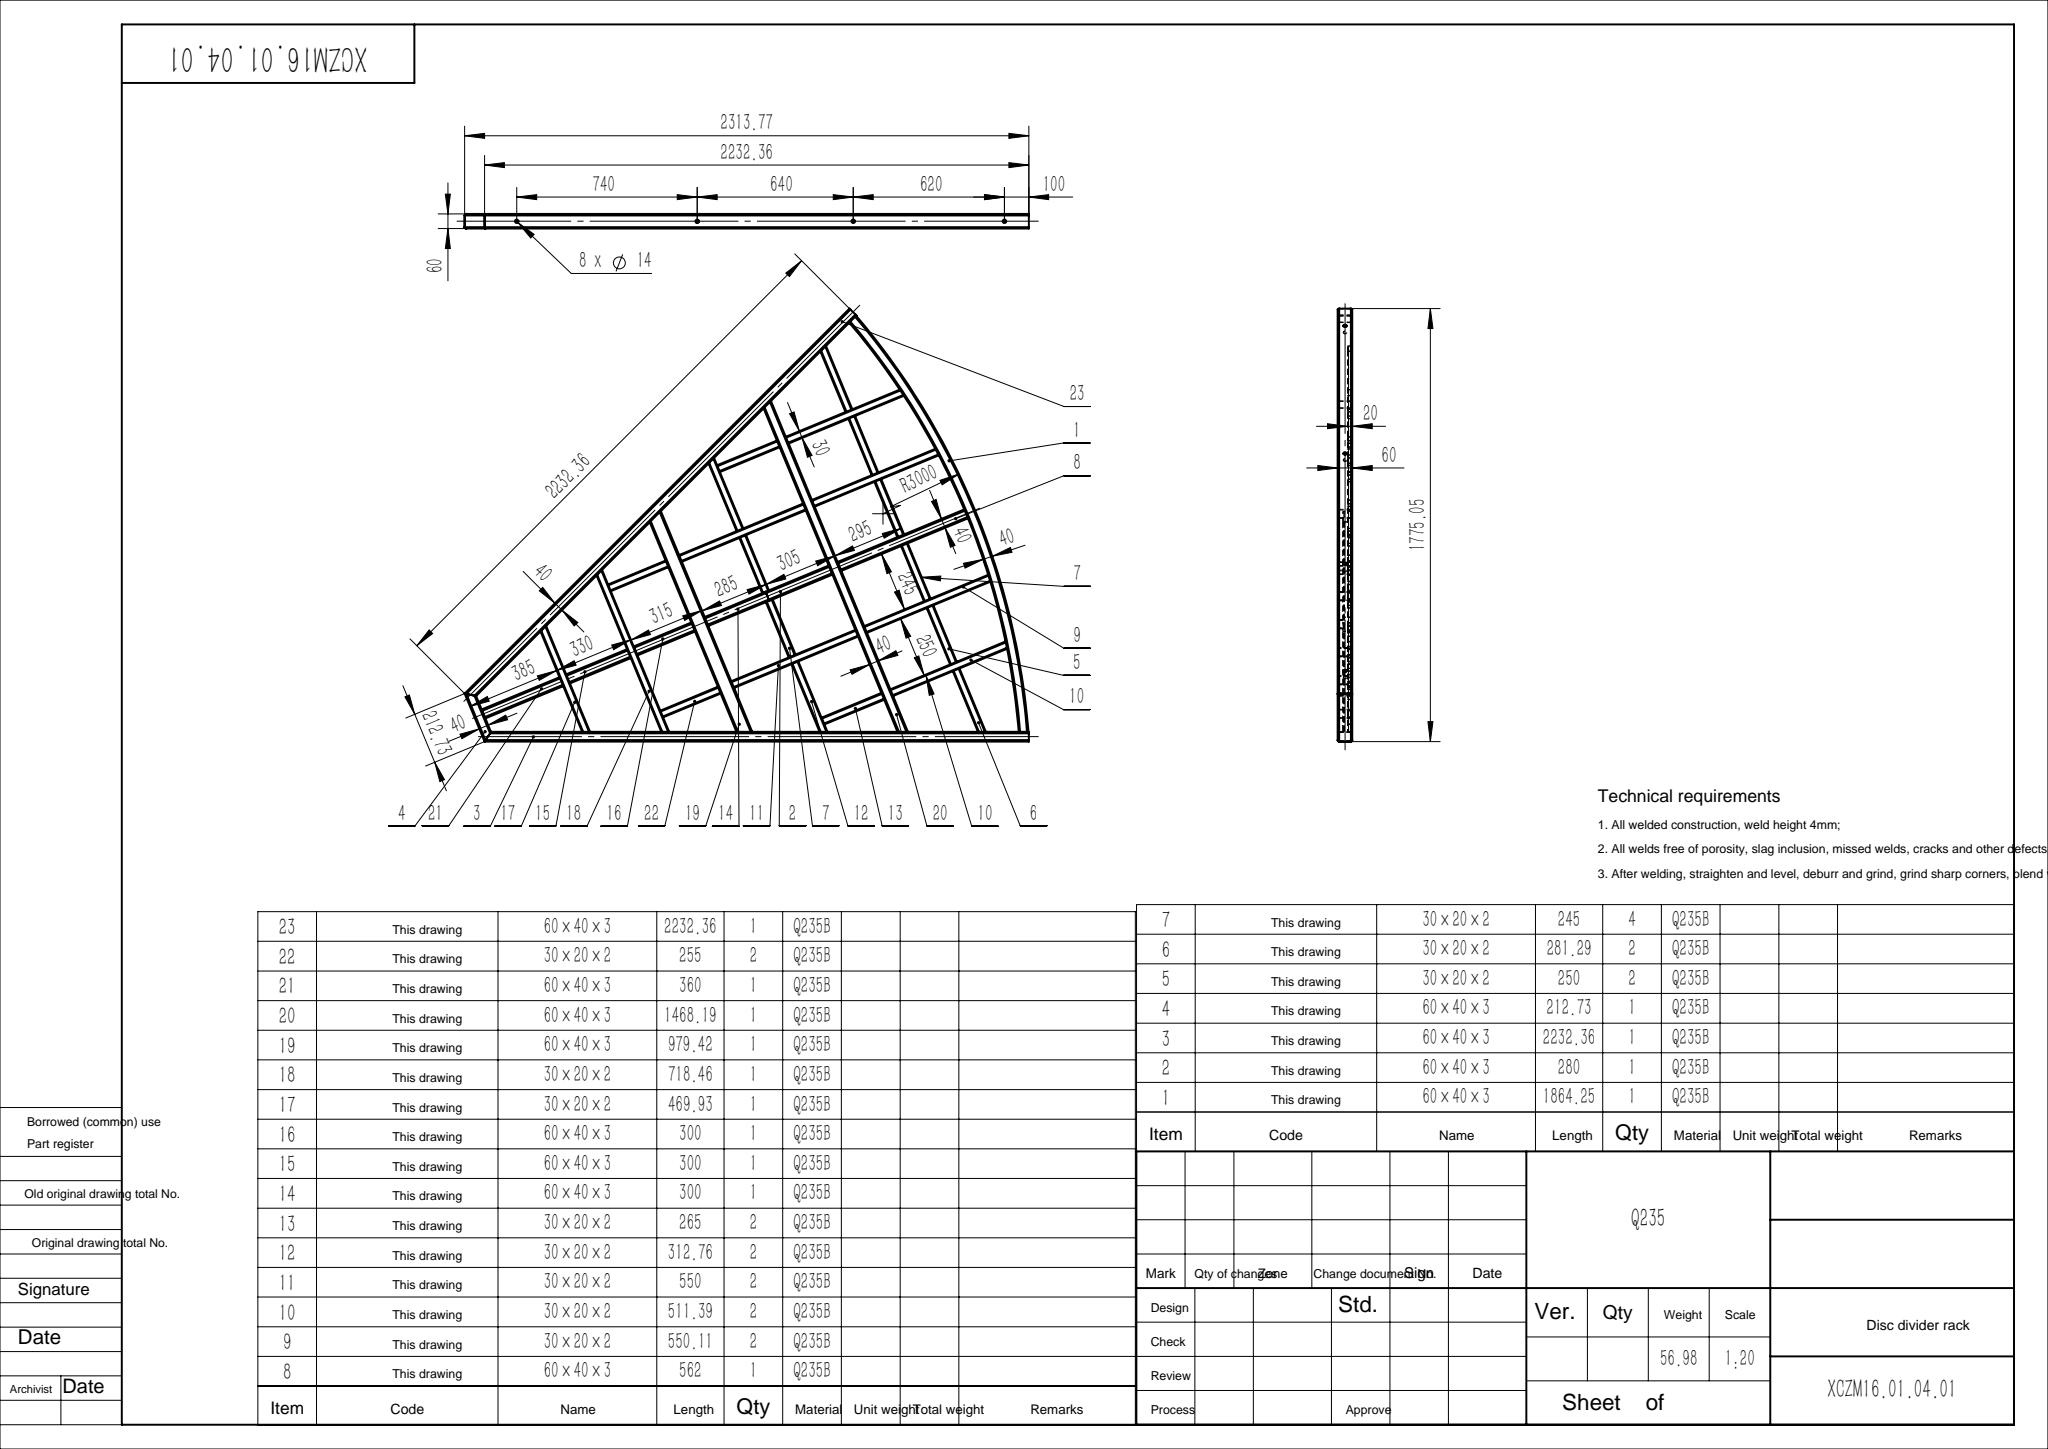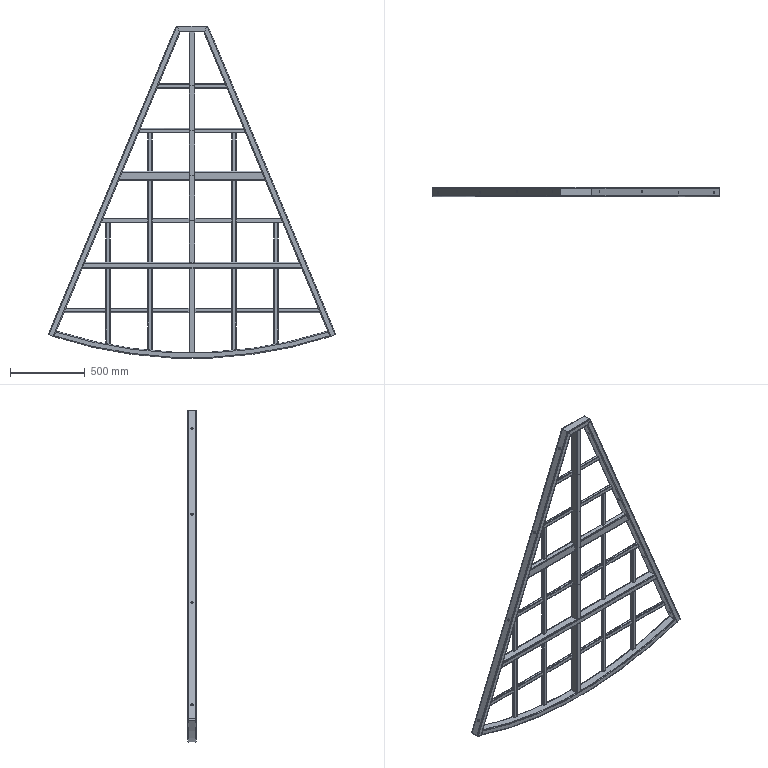Part | SolidWorks | features WeldCornerFeat 13, WeldMemberFeat 5, HoleWzd 2, WeldmentFeature 1 | 34 solids | 662 faces | box 1921 x 60 x 2222 mm | volume 7305764 mm3 | plane 349 | cylinder 305 | torus 8 | commonest cylinder face diameters 4 x88 8 x88 6 x44 12 x44 14 x32 5920 x6